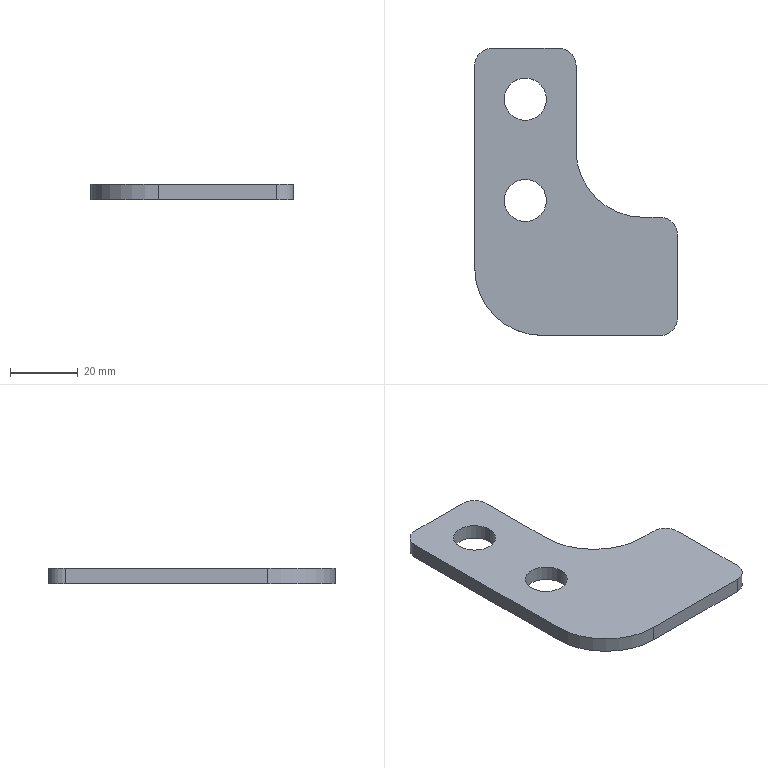Part | SolidWorks | features Extrusion 1 | 1 solid | 18 faces | box 60 x 85 x 4.5 mm | volume 14999 mm3 | cylinder 10 | plane 8 | commonest cylinder face diameters 10 x4 12.5 x4 40 x2
STEP:
#1=CARTESIAN_POINT('',(8.75,70.,4.5));
#2=VERTEX_POINT('',#1);
#3=CARTESIAN_POINT('',(21.25,70.,4.5));
#4=VERTEX_POINT('',#3);
#5=CARTESIAN_POINT('',(15.,70.,4.5));
#6=DIRECTION('',(0.,0.,1.));
#7=DIRECTION('',(1.,0.,0.));
#8=AXIS2_PLACEMENT_3D('',#5,#6,#7);
#9=CIRCLE('',#8,6.25);
#10=EDGE_CURVE('',#2,#4,#9,.T.);
#11=ORIENTED_EDGE('',*,*,#10,.T.);
#12=CARTESIAN_POINT('',(21.25,70.,0.));
#13=VERTEX_POINT('',#12);
#14=CARTESIAN_POINT('',(21.25,70.,4.5));
#15=DIRECTION('',(0.,0.,-1.));
#16=VECTOR('',#15,1000.);
#17=LINE('',#14,#16);
#18=EDGE_CURVE('',#4,#13,#17,.T.);
#19=ORIENTED_EDGE('',*,*,#18,.T.);
#20=CARTESIAN_POINT('',(8.75,70.,0.));
#21=VERTEX_POINT('',#20);
#22=CARTESIAN_POINT('',(15.,70.,0.));
#23=DIRECTION('',(0.,0.,1.));
#24=DIRECTION('',(1.,0.,0.));
#25=AXIS2_PLACEMENT_3D('',#22,#23,#24);
#26=CIRCLE('',#25,6.25);
#27=EDGE_CURVE('',#21,#13,#26,.T.);
#28=ORIENTED_EDGE('',*,*,#27,.F.);
#29=CARTESIAN_POINT('',(8.75,70.,4.5));
#30=DIRECTION('',(0.,0.,-1.));
#31=VECTOR('',#30,1000.);
#32=LINE('',#29,#31);
#33=EDGE_CURVE('',#2,#21,#32,.T.);
#34=ORIENTED_EDGE('',*,*,#33,.F.);
#35=EDGE_LOOP('',(#11,#19,#28,#34));
#36=FACE_OUTER_BOUND('',#35,.T.);
#37=CARTESIAN_POINT('',(15.,70.,4.5));
#38=DIRECTION('',(0.,0.,-1.));
#39=DIRECTION('',(-1.,0.,0.));
#40=AXIS2_PLACEMENT_3D('',#37,#38,#39);
#41=CYLINDRICAL_SURFACE('',#40,6.25);
#42=ADVANCED_FACE('',(#36),#41,.F.);
#43=CARTESIAN_POINT('',(8.75,40.,4.5));
#44=VERTEX_POINT('',#43);
#45=CARTESIAN_POINT('',(21.25,40.,4.5));
#46=VERTEX_POINT('',#45);
#47=CARTESIAN_POINT('',(15.,40.,4.5));
#48=DIRECTION('',(0.,0.,1.));
#49=DIRECTION('',(1.,0.,0.));
#50=AXIS2_PLACEMENT_3D('',#47,#48,#49);
#51=CIRCLE('',#50,6.25);
#52=EDGE_CURVE('',#44,#46,#51,.T.);
#53=ORIENTED_EDGE('',*,*,#52,.T.);
#54=CARTESIAN_POINT('',(21.25,40.,0.));
#55=VERTEX_POINT('',#54);
#56=CARTESIAN_POINT('',(21.25,40.,4.5));
#57=DIRECTION('',(0.,0.,-1.));
#58=VECTOR('',#57,1000.);
#59=LINE('',#56,#58);
#60=EDGE_CURVE('',#46,#55,#59,.T.);
#61=ORIENTED_EDGE('',*,*,#60,.T.);
#62=CARTESIAN_POINT('',(8.75,40.,0.));
#63=VERTEX_POINT('',#62);
#64=CARTESIAN_POINT('',(15.,40.,0.));
#65=DIRECTION('',(0.,0.,1.));
#66=DIRECTION('',(1.,0.,0.));
#67=AXIS2_PLACEMENT_3D('',#64,#65,#66);
#68=CIRCLE('',#67,6.25);
#69=EDGE_CURVE('',#63,#55,#68,.T.);
#70=ORIENTED_EDGE('',*,*,#69,.F.);
#71=CARTESIAN_POINT('',(8.75,40.,4.5));
#72=DIRECTION('',(0.,0.,-1.));
#73=VECTOR('',#72,1000.);
#74=LINE('',#71,#73);
#75=EDGE_CURVE('',#44,#63,#74,.T.);
#76=ORIENTED_EDGE('',*,*,#75,.F.);
#77=EDGE_LOOP('',(#53,#61,#70,#76));
#78=FACE_OUTER_BOUND('',#77,.T.);
#79=CARTESIAN_POINT('',(15.,40.,4.5));
#80=DIRECTION('',(0.,0.,-1.));
#81=DIRECTION('',(-1.,0.,0.));
#82=AXIS2_PLACEMENT_3D('',#79,#80,#81);
#83=CYLINDRICAL_SURFACE('',#82,6.25);
#84=ADVANCED_FACE('',(#78),#83,.F.);
#85=CARTESIAN_POINT('',(20.,0.,0.));
#86=VERTEX_POINT('',#85);
#87=CARTESIAN_POINT('',(55.,0.,0.));
#88=VERTEX_POINT('',#87);
#89=CARTESIAN_POINT('',(0.,0.,0.));
#90=DIRECTION('',(1.,0.,0.));
#91=VECTOR('',#90,1000.);
#92=LINE('',#89,#91);
#93=EDGE_CURVE('',#86,#88,#92,.T.);
#94=ORIENTED_EDGE('',*,*,#93,.T.);
#95=CARTESIAN_POINT('',(55.,0.,4.5));
#96=VERTEX_POINT('',#95);
#97=CARTESIAN_POINT('',(55.,0.,4.5));
#98=DIRECTION('',(0.,0.,-1.));
#99=VECTOR('',#98,1000.);
#100=LINE('',#97,#99);
#101=EDGE_CURVE('',#96,#88,#100,.T.);
#102=ORIENTED_EDGE('',*,*,#101,.F.);
#103=CARTESIAN_POINT('',(20.,0.,4.5));
#104=VERTEX_POINT('',#103);
#105=CARTESIAN_POINT('',(0.,0.,4.5));
#106=DIRECTION('',(1.,0.,0.));
#107=VECTOR('',#106,1000.);
#108=LINE('',#105,#107);
#109=EDGE_CURVE('',#104,#96,#108,.T.);
#110=ORIENTED_EDGE('',*,*,#109,.F.);
#111=CARTESIAN_POINT('',(20.,0.,4.5));
#112=DIRECTION('',(0.,0.,-1.));
#113=VECTOR('',#112,1000.);
#114=LINE('',#111,#113);
#115=EDGE_CURVE('',#104,#86,#114,.T.);
#116=ORIENTED_EDGE('',*,*,#115,.T.);
#117=EDGE_LOOP('',(#94,#102,#110,#116));
#118=FACE_OUTER_BOUND('',#117,.T.);
#119=CARTESIAN_POINT('',(0.,0.,4.5));
#120=DIRECTION('',(0.,1.,0.));
#121=DIRECTION('',(0.,0.,1.));
#122=AXIS2_PLACEMENT_3D('',#119,#120,#121);
#123=PLANE('',#122);
#124=ADVANCED_FACE('',(#118),#123,.F.);
#125=CARTESIAN_POINT('',(60.,5.,0.));
#126=VERTEX_POINT('',#125);
#127=CARTESIAN_POINT('',(55.,5.,0.));
#128=DIRECTION('',(0.,0.,1.));
#129=DIRECTION('',(1.,0.,0.));
#130=AXIS2_PLACEMENT_3D('',#127,#128,#129);
#131=CIRCLE('',#130,5.);
#132=EDGE_CURVE('',#88,#126,#131,.T.);
#133=ORIENTED_EDGE('',*,*,#132,.T.);
#134=CARTESIAN_POINT('',(60.,5.,4.5));
#135=VERTEX_POINT('',#134);
#136=CARTESIAN_POINT('',(60.,5.,4.5));
#137=DIRECTION('',(0.,0.,-1.));
#138=VECTOR('',#137,1000.);
#139=LINE('',#136,#138);
#140=EDGE_CURVE('',#135,#126,#139,.T.);
#141=ORIENTED_EDGE('',*,*,#140,.F.);
#142=CARTESIAN_POINT('',(55.,5.,4.5));
#143=DIRECTION('',(0.,0.,1.));
#144=DIRECTION('',(1.,0.,0.));
#145=AXIS2_PLACEMENT_3D('',#142,#143,#144);
#146=CIRCLE('',#145,5.);
#147=EDGE_CURVE('',#96,#135,#146,.T.);
#148=ORIENTED_EDGE('',*,*,#147,.F.);
#149=ORIENTED_EDGE('',*,*,#101,.T.);
#150=EDGE_LOOP('',(#133,#141,#148,#149));
#151=FACE_OUTER_BOUND('',#150,.T.);
#152=CARTESIAN_POINT('',(55.,5.,4.5));
#153=DIRECTION('',(0.,0.,-1.));
#154=DIRECTION('',(-1.,0.,0.));
#155=AXIS2_PLACEMENT_3D('',#152,#153,#154);
#156=CYLINDRICAL_SURFACE('',#155,5.);
#157=ADVANCED_FACE('',(#151),#156,.T.);
#158=CARTESIAN_POINT('',(60.,30.,0.));
#159=VERTEX_POINT('',#158);
#160=CARTESIAN_POINT('',(60.,0.,0.));
#161=DIRECTION('',(0.,1.,0.));
#162=VECTOR('',#161,1000.);
#163=LINE('',#160,#162);
#164=EDGE_CURVE('',#126,#159,#163,.T.);
#165=ORIENTED_EDGE('',*,*,#164,.T.);
#166=CARTESIAN_POINT('',(60.,30.,4.5));
#167=VERTEX_POINT('',#166);
#168=CARTESIAN_POINT('',(60.,30.,4.5));
#169=DIRECTION('',(0.,0.,-1.));
#170=VECTOR('',#169,1000.);
#171=LINE('',#168,#170);
#172=EDGE_CURVE('',#167,#159,#171,.T.);
#173=ORIENTED_EDGE('',*,*,#172,.F.);
#174=CARTESIAN_POINT('',(60.,0.,4.5));
#175=DIRECTION('',(0.,1.,0.));
#176=VECTOR('',#175,1000.);
#177=LINE('',#174,#176);
#178=EDGE_CURVE('',#135,#167,#177,.T.);
#179=ORIENTED_EDGE('',*,*,#178,.F.);
#180=ORIENTED_EDGE('',*,*,#140,.T.);
#181=EDGE_LOOP('',(#165,#173,#179,#180));
#182=FACE_OUTER_BOUND('',#181,.T.);
#183=CARTESIAN_POINT('',(60.,0.,4.5));
#184=DIRECTION('',(-1.,0.,0.));
#185=DIRECTION('',(0.,0.,1.));
#186=AXIS2_PLACEMENT_3D('',#183,#184,#185);
#187=PLANE('',#186);
#188=ADVANCED_FACE('',(#182),#187,.F.);
#189=CARTESIAN_POINT('',(55.,35.,0.));
#190=VERTEX_POINT('',#189);
#191=CARTESIAN_POINT('',(55.,30.,0.));
#192=DIRECTION('',(0.,0.,-1.));
#193=DIRECTION('',(1.,0.,0.));
#194=AXIS2_PLACEMENT_3D('',#191,#192,#193);
#195=CIRCLE('',#194,5.);
#196=EDGE_CURVE('',#190,#159,#195,.T.);
#197=ORIENTED_EDGE('',*,*,#196,.F.);
#198=CARTESIAN_POINT('',(55.,35.,4.5));
#199=VERTEX_POINT('',#198);
#200=CARTESIAN_POINT('',(55.,35.,4.5));
#201=DIRECTION('',(0.,0.,-1.));
#202=VECTOR('',#201,1000.);
#203=LINE('',#200,#202);
#204=EDGE_CURVE('',#199,#190,#203,.T.);
#205=ORIENTED_EDGE('',*,*,#204,.F.);
#206=CARTESIAN_POINT('',(55.,30.,4.5));
#207=DIRECTION('',(0.,0.,-1.));
#208=DIRECTION('',(1.,0.,0.));
#209=AXIS2_PLACEMENT_3D('',#206,#207,#208);
#210=CIRCLE('',#209,5.);
#211=EDGE_CURVE('',#199,#167,#210,.T.);
#212=ORIENTED_EDGE('',*,*,#211,.T.);
#213=ORIENTED_EDGE('',*,*,#172,.T.);
#214=EDGE_LOOP('',(#197,#205,#212,#213));
#215=FACE_OUTER_BOUND('',#214,.T.);
#216=CARTESIAN_POINT('',(55.,30.,4.5));
#217=DIRECTION('',(0.,0.,-1.));
#218=DIRECTION('',(-1.,0.,0.));
#219=AXIS2_PLACEMENT_3D('',#216,#217,#218);
#220=CYLINDRICAL_SURFACE('',#219,5.);
#221=ADVANCED_FACE('',(#215),#220,.T.);
#222=CARTESIAN_POINT('',(50.,35.,0.));
#223=VERTEX_POINT('',#222);
#224=CARTESIAN_POINT('',(0.,35.,0.));
#225=DIRECTION('',(1.,0.,0.));
#226=VECTOR('',#225,1000.);
#227=LINE('',#224,#226);
#228=EDGE_CURVE('',#223,#190,#227,.T.);
#229=ORIENTED_EDGE('',*,*,#228,.F.);
#230=CARTESIAN_POINT('',(50.,35.,4.5));
#231=VERTEX_POINT('',#230);
#232=CARTESIAN_POINT('',(50.,35.,4.5));
#233=DIRECTION('',(0.,0.,-1.));
#234=VECTOR('',#233,1000.);
#235=LINE('',#232,#234);
#236=EDGE_CURVE('',#231,#223,#235,.T.);
#237=ORIENTED_EDGE('',*,*,#236,.F.);
#238=CARTESIAN_POINT('',(0.,35.,4.5));
#239=DIRECTION('',(1.,0.,0.));
#240=VECTOR('',#239,1000.);
#241=LINE('',#238,#240);
#242=EDGE_CURVE('',#231,#199,#241,.T.);
#243=ORIENTED_EDGE('',*,*,#242,.T.);
#244=ORIENTED_EDGE('',*,*,#204,.T.);
#245=EDGE_LOOP('',(#229,#237,#243,#244));
#246=FACE_OUTER_BOUND('',#245,.T.);
#247=CARTESIAN_POINT('',(0.,35.,4.5));
#248=DIRECTION('',(0.,1.,0.));
#249=DIRECTION('',(0.,0.,1.));
#250=AXIS2_PLACEMENT_3D('',#247,#248,#249);
#251=PLANE('',#250);
#252=ADVANCED_FACE('',(#246),#251,.T.);
#253=CARTESIAN_POINT('',(30.,55.,0.));
#254=VERTEX_POINT('',#253);
#255=CARTESIAN_POINT('',(50.,55.,0.));
#256=DIRECTION('',(0.,0.,1.));
#257=DIRECTION('',(1.,0.,0.));
#258=AXIS2_PLACEMENT_3D('',#255,#256,#257);
#259=CIRCLE('',#258,20.);
#260=EDGE_CURVE('',#254,#223,#259,.T.);
#261=ORIENTED_EDGE('',*,*,#260,.F.);
#262=CARTESIAN_POINT('',(30.,55.,4.5));
#263=VERTEX_POINT('',#262);
#264=CARTESIAN_POINT('',(30.,55.,4.5));
#265=DIRECTION('',(0.,0.,-1.));
#266=VECTOR('',#265,1000.);
#267=LINE('',#264,#266);
#268=EDGE_CURVE('',#263,#254,#267,.T.);
#269=ORIENTED_EDGE('',*,*,#268,.F.);
#270=CARTESIAN_POINT('',(50.,55.,4.5));
#271=DIRECTION('',(0.,0.,1.));
#272=DIRECTION('',(1.,0.,0.));
#273=AXIS2_PLACEMENT_3D('',#270,#271,#272);
#274=CIRCLE('',#273,20.);
#275=EDGE_CURVE('',#263,#231,#274,.T.);
#276=ORIENTED_EDGE('',*,*,#275,.T.);
#277=ORIENTED_EDGE('',*,*,#236,.T.);
#278=EDGE_LOOP('',(#261,#269,#276,#277));
#279=FACE_OUTER_BOUND('',#278,.T.);
#280=CARTESIAN_POINT('',(50.,55.,4.5));
#281=DIRECTION('',(0.,0.,-1.));
#282=DIRECTION('',(-1.,0.,0.));
#283=AXIS2_PLACEMENT_3D('',#280,#281,#282);
#284=CYLINDRICAL_SURFACE('',#283,20.);
#285=ADVANCED_FACE('',(#279),#284,.F.);
#286=CARTESIAN_POINT('',(30.,80.,0.));
#287=VERTEX_POINT('',#286);
#288=CARTESIAN_POINT('',(30.,0.,0.));
#289=DIRECTION('',(0.,-1.,0.));
#290=VECTOR('',#289,1000.);
#291=LINE('',#288,#290);
#292=EDGE_CURVE('',#287,#254,#291,.T.);
#293=ORIENTED_EDGE('',*,*,#292,.F.);
#294=CARTESIAN_POINT('',(30.,80.,4.5));
#295=VERTEX_POINT('',#294);
#296=CARTESIAN_POINT('',(30.,80.,4.5));
#297=DIRECTION('',(0.,0.,-1.));
#298=VECTOR('',#297,1000.);
#299=LINE('',#296,#298);
#300=EDGE_CURVE('',#295,#287,#299,.T.);
#301=ORIENTED_EDGE('',*,*,#300,.F.);
#302=CARTESIAN_POINT('',(30.,0.,4.5));
#303=DIRECTION('',(0.,-1.,0.));
#304=VECTOR('',#303,1000.);
#305=LINE('',#302,#304);
#306=EDGE_CURVE('',#295,#263,#305,.T.);
#307=ORIENTED_EDGE('',*,*,#306,.T.);
#308=ORIENTED_EDGE('',*,*,#268,.T.);
#309=EDGE_LOOP('',(#293,#301,#307,#308));
#310=FACE_OUTER_BOUND('',#309,.T.);
#311=CARTESIAN_POINT('',(30.,0.,4.5));
#312=DIRECTION('',(1.,0.,0.));
#313=DIRECTION('',(0.,0.,-1.));
#314=AXIS2_PLACEMENT_3D('',#311,#312,#313);
#315=PLANE('',#314);
#316=ADVANCED_FACE('',(#310),#315,.T.);
#317=CARTESIAN_POINT('',(25.,85.,0.));
#318=VERTEX_POINT('',#317);
#319=CARTESIAN_POINT('',(25.,80.,0.));
#320=DIRECTION('',(0.,0.,-1.));
#321=DIRECTION('',(1.,0.,0.));
#322=AXIS2_PLACEMENT_3D('',#319,#320,#321);
#323=CIRCLE('',#322,5.);
#324=EDGE_CURVE('',#318,#287,#323,.T.);
#325=ORIENTED_EDGE('',*,*,#324,.F.);
#326=CARTESIAN_POINT('',(25.,85.,4.5));
#327=VERTEX_POINT('',#326);
#328=CARTESIAN_POINT('',(25.,85.,4.5));
#329=DIRECTION('',(0.,0.,-1.));
#330=VECTOR('',#329,1000.);
#331=LINE('',#328,#330);
#332=EDGE_CURVE('',#327,#318,#331,.T.);
#333=ORIENTED_EDGE('',*,*,#332,.F.);
#334=CARTESIAN_POINT('',(25.,80.,4.5));
#335=DIRECTION('',(0.,0.,-1.));
#336=DIRECTION('',(1.,0.,0.));
#337=AXIS2_PLACEMENT_3D('',#334,#335,#336);
#338=CIRCLE('',#337,5.);
#339=EDGE_CURVE('',#327,#295,#338,.T.);
#340=ORIENTED_EDGE('',*,*,#339,.T.);
#341=ORIENTED_EDGE('',*,*,#300,.T.);
#342=EDGE_LOOP('',(#325,#333,#340,#341));
#343=FACE_OUTER_BOUND('',#342,.T.);
#344=CARTESIAN_POINT('',(25.,80.,4.5));
#345=DIRECTION('',(0.,0.,-1.));
#346=DIRECTION('',(-1.,0.,0.));
#347=AXIS2_PLACEMENT_3D('',#344,#345,#346);
#348=CYLINDRICAL_SURFACE('',#347,5.);
#349=ADVANCED_FACE('',(#343),#348,.T.);
#350=CARTESIAN_POINT('',(5.,85.,0.));
#351=VERTEX_POINT('',#350);
#352=CARTESIAN_POINT('',(0.,85.,0.));
#353=DIRECTION('',(1.,0.,0.));
#354=VECTOR('',#353,1000.);
#355=LINE('',#352,#354);
#356=EDGE_CURVE('',#351,#318,#355,.T.);
#357=ORIENTED_EDGE('',*,*,#356,.F.);
#358=CARTESIAN_POINT('',(5.,85.,4.5));
#359=VERTEX_POINT('',#358);
#360=CARTESIAN_POINT('',(5.,85.,4.5));
#361=DIRECTION('',(0.,0.,-1.));
#362=VECTOR('',#361,1000.);
#363=LINE('',#360,#362);
#364=EDGE_CURVE('',#359,#351,#363,.T.);
#365=ORIENTED_EDGE('',*,*,#364,.F.);
#366=CARTESIAN_POINT('',(0.,85.,4.5));
#367=DIRECTION('',(1.,0.,0.));
#368=VECTOR('',#367,1000.);
#369=LINE('',#366,#368);
#370=EDGE_CURVE('',#359,#327,#369,.T.);
#371=ORIENTED_EDGE('',*,*,#370,.T.);
#372=ORIENTED_EDGE('',*,*,#332,.T.);
#373=EDGE_LOOP('',(#357,#365,#371,#372));
#374=FACE_OUTER_BOUND('',#373,.T.);
#375=CARTESIAN_POINT('',(0.,85.,4.5));
#376=DIRECTION('',(0.,1.,0.));
#377=DIRECTION('',(0.,0.,1.));
#378=AXIS2_PLACEMENT_3D('',#375,#376,#377);
#379=PLANE('',#378);
#380=ADVANCED_FACE('',(#374),#379,.T.);
#381=CARTESIAN_POINT('',(0.,80.,0.));
#382=VERTEX_POINT('',#381);
#383=CARTESIAN_POINT('',(5.,80.,0.));
#384=DIRECTION('',(0.,0.,-1.));
#385=DIRECTION('',(1.,0.,0.));
#386=AXIS2_PLACEMENT_3D('',#383,#384,#385);
#387=CIRCLE('',#386,5.);
#388=EDGE_CURVE('',#382,#351,#387,.T.);
#389=ORIENTED_EDGE('',*,*,#388,.F.);
#390=CARTESIAN_POINT('',(0.,80.,4.5));
#391=VERTEX_POINT('',#390);
#392=CARTESIAN_POINT('',(0.,80.,4.5));
#393=DIRECTION('',(0.,0.,-1.));
#394=VECTOR('',#393,1000.);
#395=LINE('',#392,#394);
#396=EDGE_CURVE('',#391,#382,#395,.T.);
#397=ORIENTED_EDGE('',*,*,#396,.F.);
#398=CARTESIAN_POINT('',(5.,80.,4.5));
#399=DIRECTION('',(0.,0.,-1.));
#400=DIRECTION('',(1.,0.,0.));
#401=AXIS2_PLACEMENT_3D('',#398,#399,#400);
#402=CIRCLE('',#401,5.);
#403=EDGE_CURVE('',#391,#359,#402,.T.);
#404=ORIENTED_EDGE('',*,*,#403,.T.);
#405=ORIENTED_EDGE('',*,*,#364,.T.);
#406=EDGE_LOOP('',(#389,#397,#404,#405));
#407=FACE_OUTER_BOUND('',#406,.T.);
#408=CARTESIAN_POINT('',(5.,80.,4.5));
#409=DIRECTION('',(0.,0.,-1.));
#410=DIRECTION('',(-1.,0.,0.));
#411=AXIS2_PLACEMENT_3D('',#408,#409,#410);
#412=CYLINDRICAL_SURFACE('',#411,5.);
#413=ADVANCED_FACE('',(#407),#412,.T.);
#414=CARTESIAN_POINT('',(0.,20.,0.));
#415=VERTEX_POINT('',#414);
#416=CARTESIAN_POINT('',(0.,0.,0.));
#417=DIRECTION('',(0.,1.,0.));
#418=VECTOR('',#417,1000.);
#419=LINE('',#416,#418);
#420=EDGE_CURVE('',#415,#382,#419,.T.);
#421=ORIENTED_EDGE('',*,*,#420,.F.);
#422=CARTESIAN_POINT('',(0.,20.,4.5));
#423=VERTEX_POINT('',#422);
#424=CARTESIAN_POINT('',(0.,20.,4.5));
#425=DIRECTION('',(0.,0.,-1.));
#426=VECTOR('',#425,1000.);
#427=LINE('',#424,#426);
#428=EDGE_CURVE('',#423,#415,#427,.T.);
#429=ORIENTED_EDGE('',*,*,#428,.F.);
#430=CARTESIAN_POINT('',(0.,0.,4.5));
#431=DIRECTION('',(0.,1.,0.));
#432=VECTOR('',#431,1000.);
#433=LINE('',#430,#432);
#434=EDGE_CURVE('',#423,#391,#433,.T.);
#435=ORIENTED_EDGE('',*,*,#434,.T.);
#436=ORIENTED_EDGE('',*,*,#396,.T.);
#437=EDGE_LOOP('',(#421,#429,#435,#436));
#438=FACE_OUTER_BOUND('',#437,.T.);
#439=CARTESIAN_POINT('',(0.,0.,4.5));
#440=DIRECTION('',(-1.,0.,0.));
#441=DIRECTION('',(0.,0.,1.));
#442=AXIS2_PLACEMENT_3D('',#439,#440,#441);
#443=PLANE('',#442);
#444=ADVANCED_FACE('',(#438),#443,.T.);
#445=ORIENTED_EDGE('',*,*,#60,.F.);
#446=CARTESIAN_POINT('',(15.,40.,4.5));
#447=DIRECTION('',(0.,0.,1.));
#448=DIRECTION('',(1.,0.,0.));
#449=AXIS2_PLACEMENT_3D('',#446,#447,#448);
#450=CIRCLE('',#449,6.25);
#451=EDGE_CURVE('',#46,#44,#450,.T.);
#452=ORIENTED_EDGE('',*,*,#451,.T.);
#453=ORIENTED_EDGE('',*,*,#75,.T.);
#454=CARTESIAN_POINT('',(15.,40.,0.));
#455=DIRECTION('',(0.,0.,1.));
#456=DIRECTION('',(1.,0.,0.));
#457=AXIS2_PLACEMENT_3D('',#454,#455,#456);
#458=CIRCLE('',#457,6.25);
#459=EDGE_CURVE('',#55,#63,#458,.T.);
#460=ORIENTED_EDGE('',*,*,#459,.F.);
#461=EDGE_LOOP('',(#445,#452,#453,#460));
#462=FACE_OUTER_BOUND('',#461,.T.);
#463=CARTESIAN_POINT('',(15.,40.,4.5));
#464=DIRECTION('',(0.,0.,-1.));
#465=DIRECTION('',(-1.,0.,0.));
#466=AXIS2_PLACEMENT_3D('',#463,#464,#465);
#467=CYLINDRICAL_SURFACE('',#466,6.25);
#468=ADVANCED_FACE('',(#462),#467,.F.);
#469=ORIENTED_EDGE('',*,*,#18,.F.);
#470=CARTESIAN_POINT('',(15.,70.,4.5));
#471=DIRECTION('',(0.,0.,1.));
#472=DIRECTION('',(1.,0.,0.));
#473=AXIS2_PLACEMENT_3D('',#470,#471,#472);
#474=CIRCLE('',#473,6.25);
#475=EDGE_CURVE('',#4,#2,#474,.T.);
#476=ORIENTED_EDGE('',*,*,#475,.T.);
#477=ORIENTED_EDGE('',*,*,#33,.T.);
#478=CARTESIAN_POINT('',(15.,70.,0.));
#479=DIRECTION('',(0.,0.,1.));
#480=DIRECTION('',(1.,0.,0.));
#481=AXIS2_PLACEMENT_3D('',#478,#479,#480);
#482=CIRCLE('',#481,6.25);
#483=EDGE_CURVE('',#13,#21,#482,.T.);
#484=ORIENTED_EDGE('',*,*,#483,.F.);
#485=EDGE_LOOP('',(#469,#476,#477,#484));
#486=FACE_OUTER_BOUND('',#485,.T.);
#487=CARTESIAN_POINT('',(15.,70.,4.5));
#488=DIRECTION('',(0.,0.,-1.));
#489=DIRECTION('',(-1.,0.,0.));
#490=AXIS2_PLACEMENT_3D('',#487,#488,#489);
#491=CYLINDRICAL_SURFACE('',#490,6.25);
#492=ADVANCED_FACE('',(#486),#491,.F.);
#493=CARTESIAN_POINT('',(20.,20.,0.));
#494=DIRECTION('',(0.,0.,-1.));
#495=DIRECTION('',(1.,0.,0.));
#496=AXIS2_PLACEMENT_3D('',#493,#494,#495);
#497=CIRCLE('',#496,20.);
#498=EDGE_CURVE('',#86,#415,#497,.T.);
#499=ORIENTED_EDGE('',*,*,#498,.F.);
#500=ORIENTED_EDGE('',*,*,#115,.F.);
#501=CARTESIAN_POINT('',(20.,20.,4.5));
#502=DIRECTION('',(0.,0.,-1.));
#503=DIRECTION('',(1.,0.,0.));
#504=AXIS2_PLACEMENT_3D('',#501,#502,#503);
#505=CIRCLE('',#504,20.);
#506=EDGE_CURVE('',#104,#423,#505,.T.);
#507=ORIENTED_EDGE('',*,*,#506,.T.);
#508=ORIENTED_EDGE('',*,*,#428,.T.);
#509=EDGE_LOOP('',(#499,#500,#507,#508));
#510=FACE_OUTER_BOUND('',#509,.T.);
#511=CARTESIAN_POINT('',(20.,20.,4.5));
#512=DIRECTION('',(0.,0.,-1.));
#513=DIRECTION('',(-1.,0.,0.));
#514=AXIS2_PLACEMENT_3D('',#511,#512,#513);
#515=CYLINDRICAL_SURFACE('',#514,20.);
#516=ADVANCED_FACE('',(#510),#515,.T.);
#517=ORIENTED_EDGE('',*,*,#10,.F.);
#518=ORIENTED_EDGE('',*,*,#475,.F.);
#519=EDGE_LOOP('',(#517,#518));
#520=FACE_BOUND('',#519,.T.);
#521=ORIENTED_EDGE('',*,*,#52,.F.);
#522=ORIENTED_EDGE('',*,*,#451,.F.);
#523=EDGE_LOOP('',(#521,#522));
#524=FACE_BOUND('',#523,.T.);
#525=ORIENTED_EDGE('',*,*,#109,.T.);
#526=ORIENTED_EDGE('',*,*,#147,.T.);
#527=ORIENTED_EDGE('',*,*,#178,.T.);
#528=ORIENTED_EDGE('',*,*,#211,.F.);
#529=ORIENTED_EDGE('',*,*,#242,.F.);
#530=ORIENTED_EDGE('',*,*,#275,.F.);
#531=ORIENTED_EDGE('',*,*,#306,.F.);
#532=ORIENTED_EDGE('',*,*,#339,.F.);
#533=ORIENTED_EDGE('',*,*,#370,.F.);
#534=ORIENTED_EDGE('',*,*,#403,.F.);
#535=ORIENTED_EDGE('',*,*,#434,.F.);
#536=ORIENTED_EDGE('',*,*,#506,.F.);
#537=EDGE_LOOP('',(#525,#526,#527,#528,#529,#530,#531,#532,#533,#534,#535,#536));
#538=FACE_OUTER_BOUND('',#537,.T.);
#539=CARTESIAN_POINT('',(0.,0.,4.5));
#540=DIRECTION('',(0.,0.,1.));
#541=DIRECTION('',(1.,0.,0.));
#542=AXIS2_PLACEMENT_3D('',#539,#540,#541);
#543=PLANE('',#542);
#544=ADVANCED_FACE('',(#520,#524,#538),#543,.T.);
#545=ORIENTED_EDGE('',*,*,#27,.T.);
#546=ORIENTED_EDGE('',*,*,#483,.T.);
#547=EDGE_LOOP('',(#545,#546));
#548=FACE_BOUND('',#547,.T.);
#549=ORIENTED_EDGE('',*,*,#69,.T.);
#550=ORIENTED_EDGE('',*,*,#459,.T.);
#551=EDGE_LOOP('',(#549,#550));
#552=FACE_BOUND('',#551,.T.);
#553=ORIENTED_EDGE('',*,*,#93,.F.);
#554=ORIENTED_EDGE('',*,*,#498,.T.);
#555=ORIENTED_EDGE('',*,*,#420,.T.);
#556=ORIENTED_EDGE('',*,*,#388,.T.);
#557=ORIENTED_EDGE('',*,*,#356,.T.);
#558=ORIENTED_EDGE('',*,*,#324,.T.);
#559=ORIENTED_EDGE('',*,*,#292,.T.);
#560=ORIENTED_EDGE('',*,*,#260,.T.);
#561=ORIENTED_EDGE('',*,*,#228,.T.);
#562=ORIENTED_EDGE('',*,*,#196,.T.);
#563=ORIENTED_EDGE('',*,*,#164,.F.);
#564=ORIENTED_EDGE('',*,*,#132,.F.);
#565=EDGE_LOOP('',(#553,#554,#555,#556,#557,#558,#559,#560,#561,#562,#563,#564));
#566=FACE_OUTER_BOUND('',#565,.T.);
#567=CARTESIAN_POINT('',(0.,0.,0.));
#568=DIRECTION('',(0.,0.,1.));
#569=DIRECTION('',(1.,0.,0.));
#570=AXIS2_PLACEMENT_3D('',#567,#568,#569);
#571=PLANE('',#570);
#572=ADVANCED_FACE('',(#548,#552,#566),#571,.F.);
#573=CLOSED_SHELL('',(#42,#84,#124,#157,#188,#221,#252,#285,#316,#349,#380,#413,#444,#468,#492,#516,#544,#572));
#574=MANIFOLD_SOLID_BREP('',#573);
#575=CARTESIAN_POINT('',(0.,0.,0.));
#576=DIRECTION('',(0.,0.,1.));
#577=DIRECTION('',(1.,0.,0.));
#578=AXIS2_PLACEMENT_3D('',#575,#576,#577);
#579=(LENGTH_UNIT()NAMED_UNIT(*)SI_UNIT(.MILLI.,.METRE.));
#580=UNCERTAINTY_MEASURE_WITH_UNIT(LENGTH_MEASURE(0.00001),#579,'','');
#581=(NAMED_UNIT(*)PLANE_ANGLE_UNIT()SI_UNIT($,.RADIAN.));
#582=(NAMED_UNIT(*)SI_UNIT($,.STERADIAN.)SOLID_ANGLE_UNIT());
#583=(GEOMETRIC_REPRESENTATION_CONTEXT(3)GLOBAL_UNCERTAINTY_ASSIGNED_CONTEXT((#580))GLOBAL_UNIT_ASSIGNED_CONTEXT((#579,#581,#582))REPRESENTATION_CONTEXT('',''));
#584=ADVANCED_BREP_SHAPE_REPRESENTATION('',(#574,#578),#583);